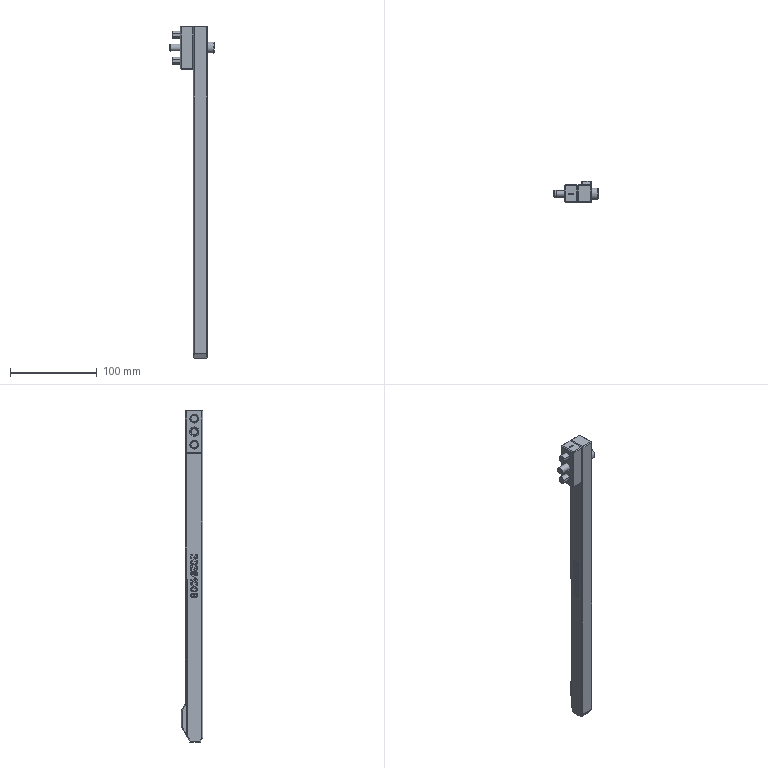Part | NX | features BREP 22, solid 10, CHAMFER 9, SUBTRACT 5 | 5 solids | 289 faces | box 51 x 25 x 382.34 mm | volume 137909 mm3 | plane 137 | spline 115 | cone 23 | cylinder 14 | commonest cylinder face diameters 8 x7 3.2 x2 4 x2 9 x2 13 x1